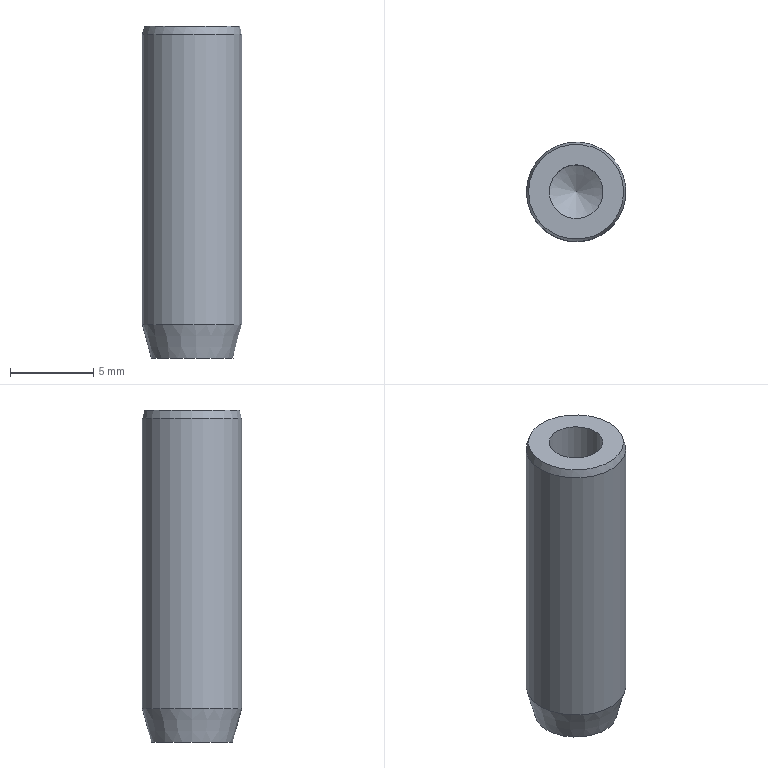Part | NX | features 5003_337_MSHT6-20 2 | 1 solid | 7 faces | box 6 x 6 x 20 mm | volume 486.645 mm3 | cone 3 | plane 2 | cylinder 2 | commonest cylinder face diameters 3.242 x1 6 x1
STEP:
#1=CARTESIAN_POINT('',(99.6,-171.379,-228.));
#2=VERTEX_POINT('',#1);
#3=CARTESIAN_POINT('',(99.6,-173.,-228.));
#4=DIRECTION('',(0.,0.,1.));
#5=DIRECTION('',(0.,1.,0.));
#6=AXIS2_PLACEMENT_3D('',#3,#4,#5);
#7=CIRCLE('',#6,1.621);
#8=EDGE_CURVE('',#2,#2,#7,.T.);
#9=ORIENTED_EDGE('',*,*,#8,.F.);
#10=EDGE_LOOP('',(#9));
#11=FACE_BOUND('',#10,.T.);
#12=CARTESIAN_POINT('',(96.734,-173.,-228.));
#13=VERTEX_POINT('',#12);
#14=CARTESIAN_POINT('',(99.6,-173.,-228.));
#15=DIRECTION('',(0.,0.,-1.));
#16=DIRECTION('',(-1.,0.,0.));
#17=AXIS2_PLACEMENT_3D('',#14,#15,#16);
#18=CIRCLE('',#17,2.866);
#19=EDGE_CURVE('',#13,#13,#18,.T.);
#20=ORIENTED_EDGE('',*,*,#19,.F.);
#21=EDGE_LOOP('',(#20));
#22=FACE_BOUND('',#21,.T.);
#23=CARTESIAN_POINT('',(99.6,-173.,-228.));
#24=DIRECTION('',(0.,0.,1.));
#25=DIRECTION('',(1.,0.,0.));
#26=AXIS2_PLACEMENT_3D('',#23,#24,#25);
#27=PLANE('',#26);
#28=ADVANCED_FACE('',(#11,#22),#27,.T.);
#29=ORIENTED_EDGE('',*,*,#19,.T.);
#30=EDGE_LOOP('',(#29));
#31=FACE_BOUND('',#30,.T.);
#32=CARTESIAN_POINT('',(96.6,-173.,-228.5));
#33=VERTEX_POINT('',#32);
#34=CARTESIAN_POINT('',(99.6,-173.,-228.5));
#35=DIRECTION('',(0.,0.,-1.));
#36=DIRECTION('',(-1.,0.,0.));
#37=AXIS2_PLACEMENT_3D('',#34,#35,#36);
#38=CIRCLE('',#37,3.);
#39=EDGE_CURVE('',#33,#33,#38,.T.);
#40=ORIENTED_EDGE('',*,*,#39,.F.);
#41=EDGE_LOOP('',(#40));
#42=FACE_BOUND('',#41,.T.);
#43=CARTESIAN_POINT('',(99.6,-173.,-228.5));
#44=DIRECTION('',(0.,0.,-1.));
#45=DIRECTION('',(-1.,0.,0.));
#46=AXIS2_PLACEMENT_3D('',#43,#44,#45);
#47=CONICAL_SURFACE('',#46,3.,0.2618);
#48=ADVANCED_FACE('',(#31,#42),#47,.T.);
#49=ORIENTED_EDGE('',*,*,#39,.T.);
#50=EDGE_LOOP('',(#49));
#51=FACE_BOUND('',#50,.T.);
#52=CARTESIAN_POINT('',(96.6,-173.,-246.));
#53=VERTEX_POINT('',#52);
#54=CARTESIAN_POINT('',(99.6,-173.,-246.));
#55=DIRECTION('',(0.,0.,-1.));
#56=DIRECTION('',(-1.,0.,0.));
#57=AXIS2_PLACEMENT_3D('',#54,#55,#56);
#58=CIRCLE('',#57,3.);
#59=EDGE_CURVE('',#53,#53,#58,.T.);
#60=ORIENTED_EDGE('',*,*,#59,.F.);
#61=EDGE_LOOP('',(#60));
#62=FACE_BOUND('',#61,.T.);
#63=CARTESIAN_POINT('',(99.6,-173.,-248.));
#64=DIRECTION('',(0.,0.,-1.));
#65=DIRECTION('',(-1.,0.,0.));
#66=AXIS2_PLACEMENT_3D('',#63,#64,#65);
#67=CYLINDRICAL_SURFACE('',#66,3.);
#68=ADVANCED_FACE('',(#51,#62),#67,.T.);
#69=ORIENTED_EDGE('',*,*,#59,.T.);
#70=EDGE_LOOP('',(#69));
#71=FACE_BOUND('',#70,.T.);
#72=CARTESIAN_POINT('',(97.136,-173.,-248.));
#73=VERTEX_POINT('',#72);
#74=CARTESIAN_POINT('',(99.6,-173.,-248.));
#75=DIRECTION('',(0.,0.,-1.));
#76=DIRECTION('',(-1.,0.,0.));
#77=AXIS2_PLACEMENT_3D('',#74,#75,#76);
#78=CIRCLE('',#77,2.464);
#79=EDGE_CURVE('',#73,#73,#78,.T.);
#80=ORIENTED_EDGE('',*,*,#79,.F.);
#81=EDGE_LOOP('',(#80));
#82=FACE_BOUND('',#81,.T.);
#83=CARTESIAN_POINT('',(99.6,-173.,-248.));
#84=DIRECTION('',(0.,0.,1.));
#85=DIRECTION('',(1.,0.,0.));
#86=AXIS2_PLACEMENT_3D('',#83,#84,#85);
#87=CONICAL_SURFACE('',#86,2.464,0.2618);
#88=ADVANCED_FACE('',(#71,#82),#87,.T.);
#89=ORIENTED_EDGE('',*,*,#79,.T.);
#90=EDGE_LOOP('',(#89));
#91=FACE_BOUND('',#90,.T.);
#92=CARTESIAN_POINT('',(99.6,-173.,-248.));
#93=DIRECTION('',(0.,0.,-1.));
#94=DIRECTION('',(-1.,0.,0.));
#95=AXIS2_PLACEMENT_3D('',#92,#93,#94);
#96=PLANE('',#95);
#97=ADVANCED_FACE('',(#91),#96,.T.);
#98=CARTESIAN_POINT('',(99.6,-173.,-236.974));
#99=VERTEX_POINT('',#98);
#100=VERTEX_LOOP('',#99);
#101=FACE_BOUND('',#100,.T.);
#102=CARTESIAN_POINT('',(99.6,-171.379,-236.));
#103=VERTEX_POINT('',#102);
#104=CARTESIAN_POINT('',(99.6,-173.,-236.));
#105=DIRECTION('',(0.,0.,1.));
#106=DIRECTION('',(0.,1.,0.));
#107=AXIS2_PLACEMENT_3D('',#104,#105,#106);
#108=CIRCLE('',#107,1.621);
#109=EDGE_CURVE('',#103,#103,#108,.T.);
#110=ORIENTED_EDGE('',*,*,#109,.T.);
#111=EDGE_LOOP('',(#110));
#112=FACE_BOUND('',#111,.T.);
#113=CARTESIAN_POINT('',(99.6,-173.,-236.));
#114=DIRECTION('',(0.,0.,1.));
#115=DIRECTION('',(0.,1.,0.));
#116=AXIS2_PLACEMENT_3D('',#113,#114,#115);
#117=CONICAL_SURFACE('',#116,1.621,1.03);
#118=ADVANCED_FACE('',(#101,#112),#117,.F.);
#119=ORIENTED_EDGE('',*,*,#109,.F.);
#120=EDGE_LOOP('',(#119));
#121=FACE_BOUND('',#120,.T.);
#122=ORIENTED_EDGE('',*,*,#8,.T.);
#123=EDGE_LOOP('',(#122));
#124=FACE_BOUND('',#123,.T.);
#125=CARTESIAN_POINT('',(99.6,-173.,-228.));
#126=DIRECTION('',(0.,0.,1.));
#127=DIRECTION('',(0.,1.,0.));
#128=AXIS2_PLACEMENT_3D('',#125,#126,#127);
#129=CYLINDRICAL_SURFACE('',#128,1.621);
#130=ADVANCED_FACE('',(#121,#124),#129,.F.);
#131=CLOSED_SHELL('',(#28,#48,#68,#88,#97,#118,#130));
#132=MANIFOLD_SOLID_BREP('',#131);
#133=(LENGTH_UNIT()NAMED_UNIT(*)SI_UNIT(.MILLI.,.METRE.));
#134=UNCERTAINTY_MEASURE_WITH_UNIT(LENGTH_MEASURE(0.00001),#133,'','');
#135=(NAMED_UNIT(*)PLANE_ANGLE_UNIT()SI_UNIT($,.RADIAN.));
#136=(NAMED_UNIT(*)SI_UNIT($,.STERADIAN.)SOLID_ANGLE_UNIT());
#137=(GEOMETRIC_REPRESENTATION_CONTEXT(3)GLOBAL_UNCERTAINTY_ASSIGNED_CONTEXT((#134))GLOBAL_UNIT_ASSIGNED_CONTEXT((#133,#135,#136))REPRESENTATION_CONTEXT('',''));
#138=ADVANCED_BREP_SHAPE_REPRESENTATION('',(#132),#137);